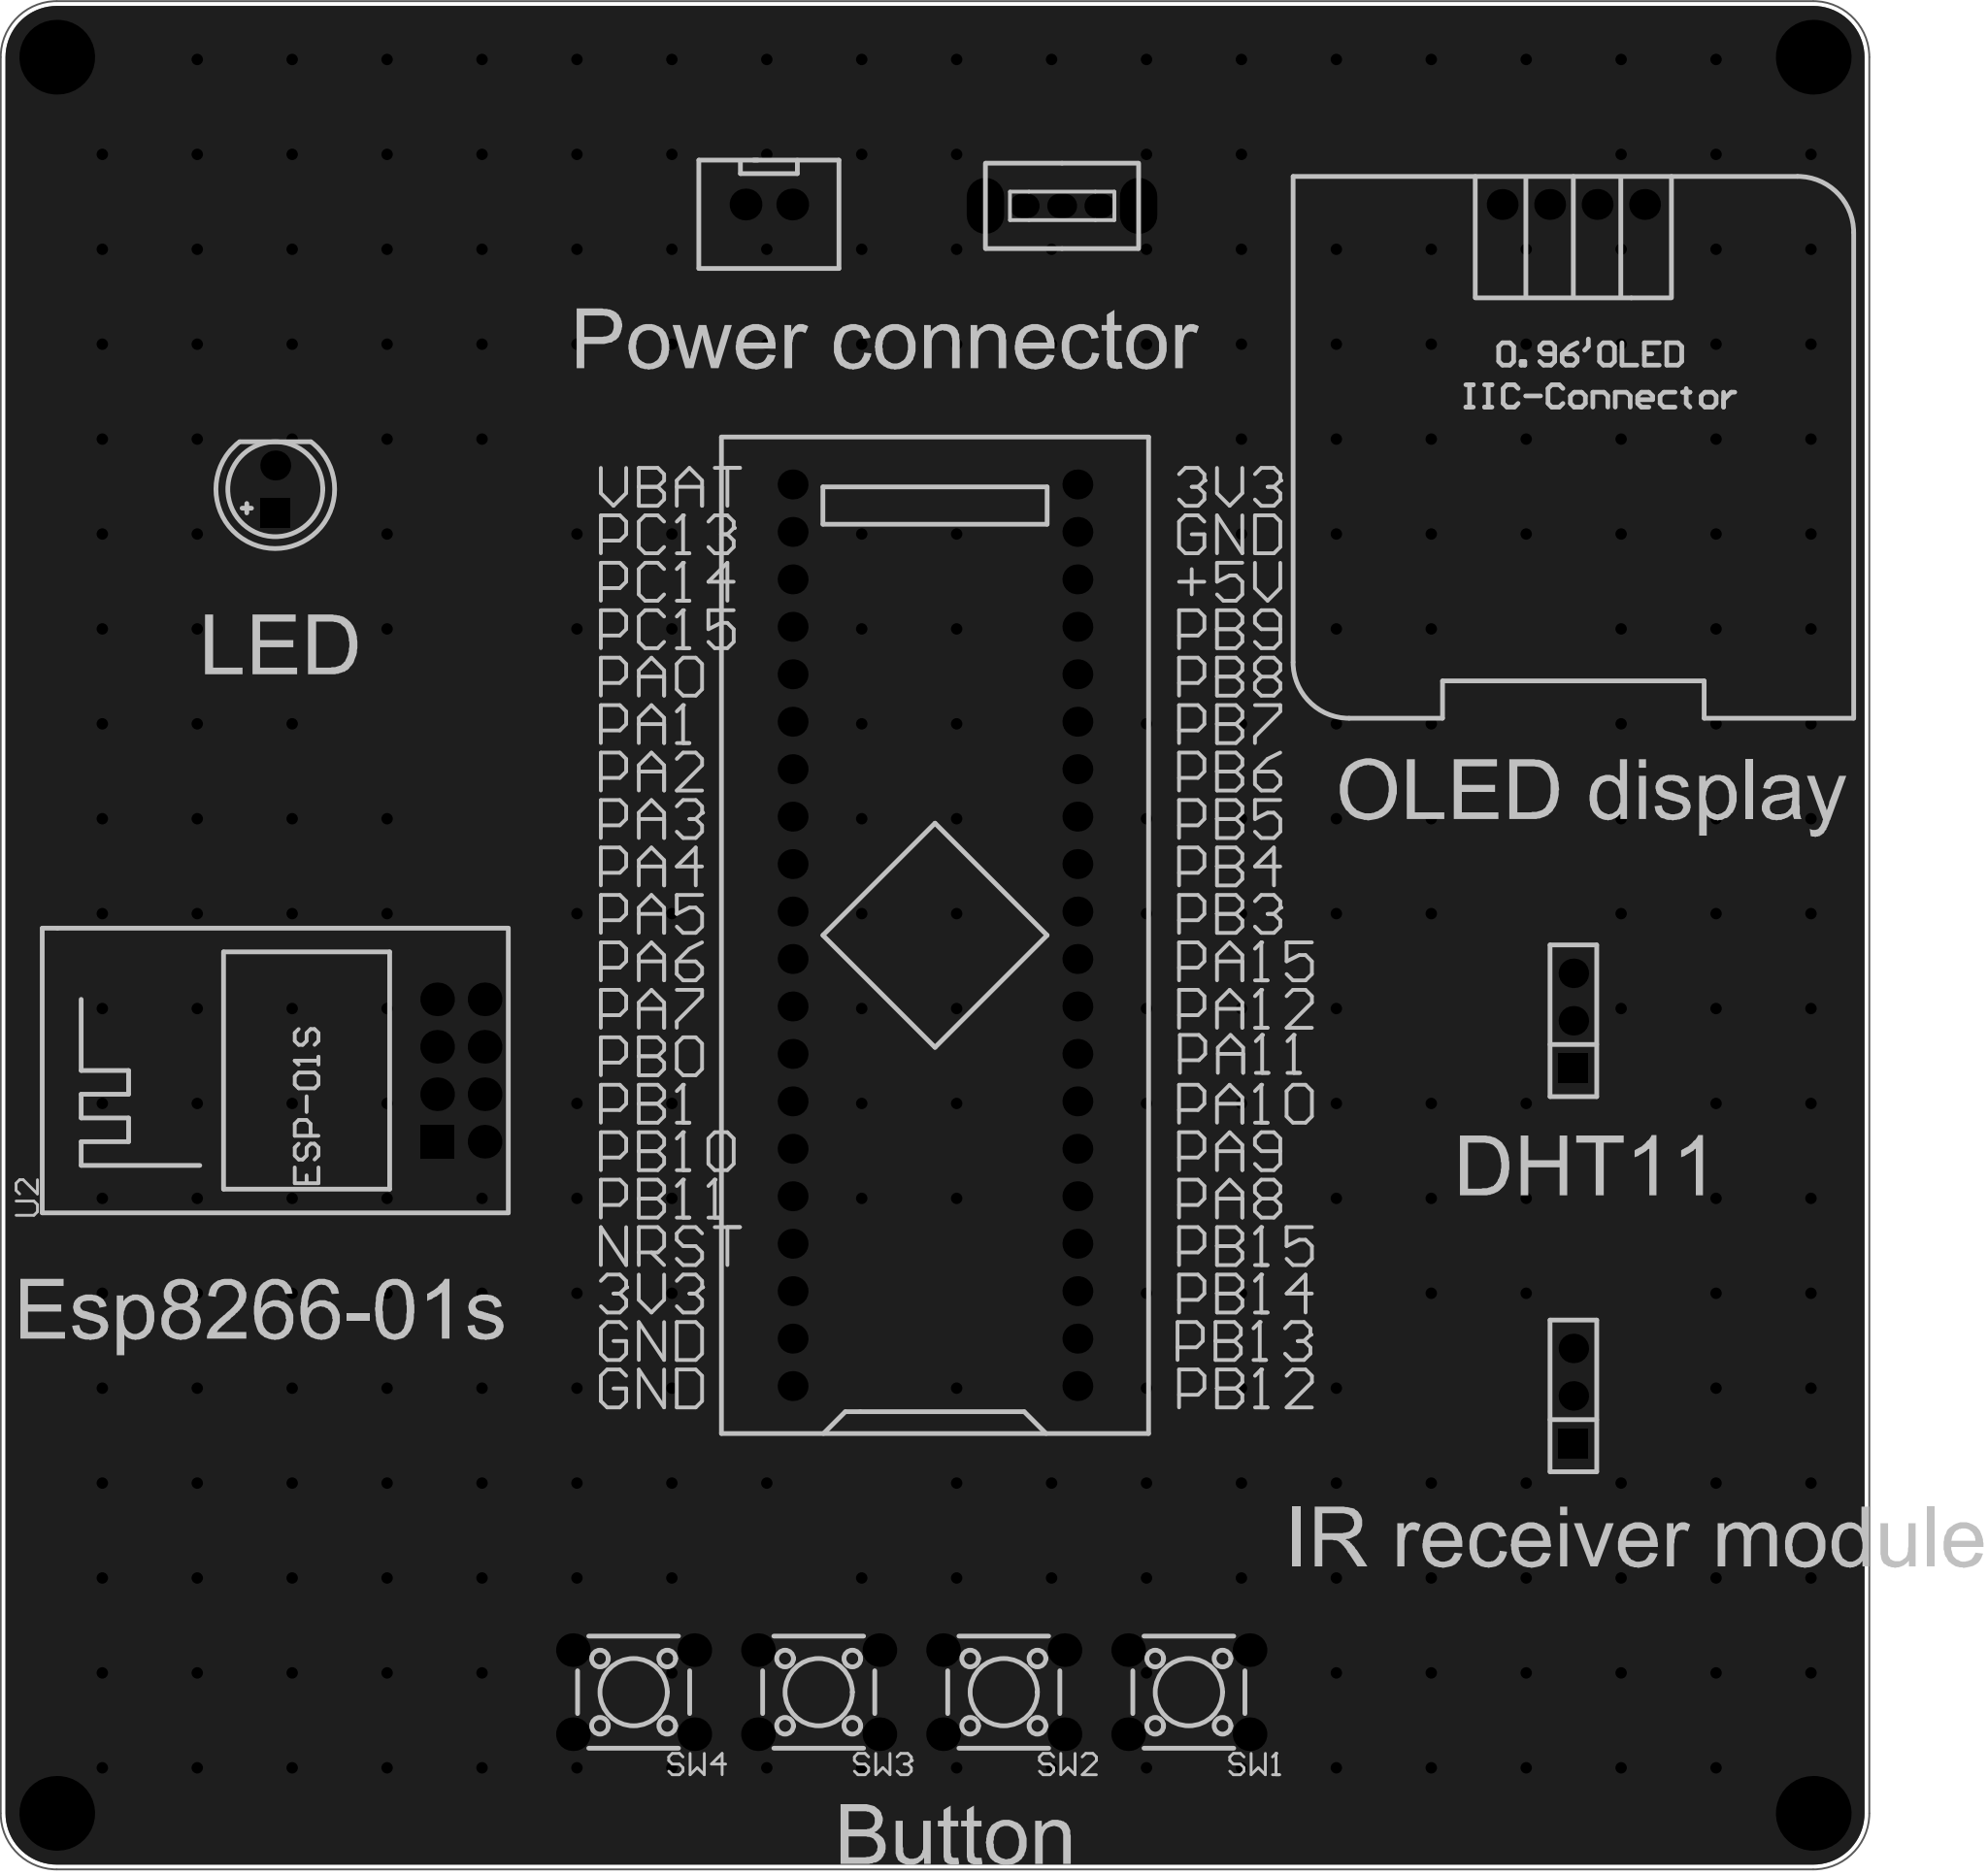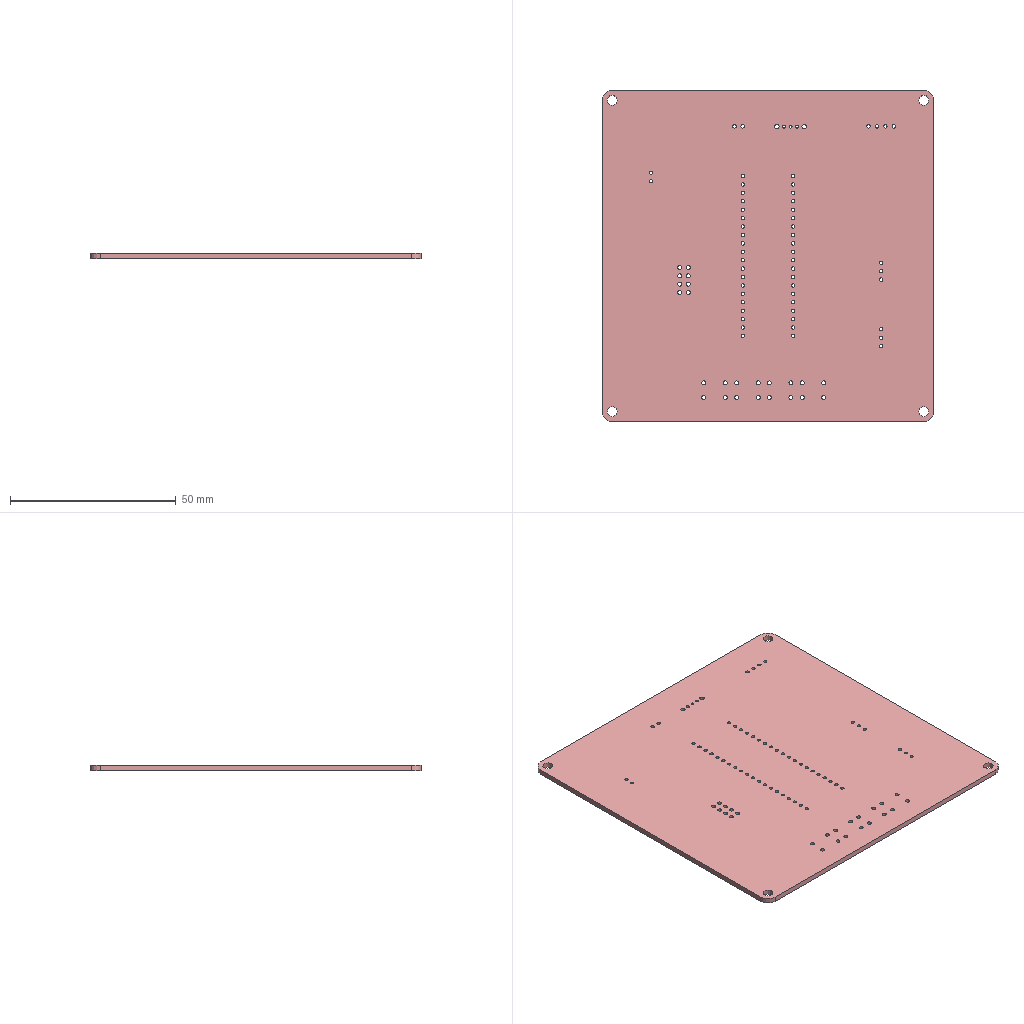Circuit board layout | Altium Designer | box 100 x 100 x 1.6 mm
Layer stack:
# Altium Designer layer stack of  (unit mm; dielectric type: 0 none, 1 core, 2 prepreg, 3 surface material)
index,name,kind,layer,copper_thickness_mm,dielectric_type,dielectric_thickness_mm,dielectric_material,dielectric_constant
0,Top Paste Mask Layer,other,,,,,,
1,Top Silkscreen Layer,other,,,,,,
2,Top Solder Mask Layer,dielectric,,,3,0.01,,3.3
3,Top Layer,copper,Top Layer,0.035,,,,
4,Dielectric1,dielectric,,,3,1.51,FR4,4.5
5,Bottom Layer,copper,Bottom Layer,0.035,,,,
6,Bottom Solder Mask Layer,dielectric,,,3,0.01,,3.3
7,Bottom Silkscreen Layer,other,,,,,,
8,Bottom Paste Mask Layer,other,,,,,,
# drill layer pairs: low layer,high layer
drill_pair,Top Layer,Bottom Layer
Part placement:
Designator,Comment,Layer,Footprint,Center-X(mm),Center-Y(mm),Rotation
U1,STM32F103C8T6-Card,TopLayer,CONN-TH_L53.3-W22.9_STM32F103C8T6-CARD,141.351,130.937,90
SW1,,TopLayer,SW-TH_4P-L6.0-W6.0-P4.50-LS6.5,154.936,90.424,180
SW2,,TopLayer,SW-TH_4P-L6.0-W6.0-P4.50-LS6.5,145.031,90.424,180
SW3,,TopLayer,SW-TH_4P-L6.0-W6.0-P4.50-LS6.5,135.127,90.424,180
SW4,,TopLayer,SW-TH_4P-L6.0-W6.0-P4.50-LS6.5,125.222,90.424,180
CN4,XH2.54*2P_THT,TopLayer,CONN-TH_2P-P2.50-XH2.54-2P,132.461,170.053,0
SW5,,TopLayer,拨动开关,148.148,169.978,180
H1,,TopLayer,HDR-TH_3P-P2.54-V-F,175.514,106.281,90
H3,,TopLayer,HDR-TH_3P-P2.54-V-F,175.514,126.36,90
LED1,,TopLayer,LED-TH_5mm,106.045,154.813,90
OLED1,,TopLayer,0.96OLED_4P,175.514,170.053,0
U2,ESP-01S,TopLayer,WIFIM-TH_ESP-01S,115.976,123.698,90
Pad and via stacks:
# Altium Designer via and pad stacks of  (unit mm). Each distinct definition once, with the count of objects using it.
# via: kind,start_layer,end_layer,hole_mm,diameter_mm,mode(0 simple;1 top-mid-bottom;2 full stack),diameter_per_layer,count,example_net
# pad: kind,layer,hole_mm,hole_type(0 round;1 square;2 slot),plating,top_size,top_shape(1 round;2 rect;3 octagon;9 rounded rect),mid_size,bottom_size,mode,footprint,size_per_layer,count,example
pad,Multi-Layer,3,0,plated,4x4,1,4x4,4x4,0,,,4,1
pad,Multi-Layer,1,0,plated,1.6x1.6,1,1.6x1.6,1.6x1.6,0,CONN-TH_L53.3-W22.9_STM32F103C8T6-CARD,,40,U1.1
pad,Multi-Layer,1.2,0,plated,1.8x1.8,1,1.8x1.8,1.8x1.8,0,SW-TH_4P-L6.0-W6.0-P4.50-LS6.5,,16,SW1.1
pad,Multi-Layer,1.05,0,plated,1.7x1.7,1,1.7x1.7,1.7x1.7,0,CONN-TH_2P-P2.50-XH2.54-2P,,2,CN4.2
pad,Multi-Layer,0.8992,0,plated,1.6x1.3,1,1.6x1.3,1.6x1.3,0,\u00B2\u00A6\u00B6\u00AF\u00BF\u00AA\u00B9\u00D8,,3,SW5.1
pad,Multi-Layer,1.3,0,plated,3x1.999,1,3x1.999,3x1.999,0,\u00B2\u00A6\u00B6\u00AF\u00BF\u00AA\u00B9\u00D8,,2,SW5.4
pad,Multi-Layer,1.02,0,plated,1.575x1.575,1,1.575x1.575,1.575x1.575,0,HDR-TH_3P-P2.54-V-F,,4,H1.3
pad,Multi-Layer,1.02,0,plated,1.575x1.575,2,1.575x1.575,1.575x1.575,0,HDR-TH_3P-P2.54-V-F,,2,H1.1
pad,Multi-Layer,1,0,plated,1.6x1.6,2,1.6x1.6,1.6x1.6,0,LED-TH_5mm,,1,LED1.1
pad,Multi-Layer,1,0,plated,1.6x1.6,1,1.6x1.6,1.6x1.6,0,LED-TH_5mm,,1,LED1.2
pad,Multi-Layer,1,0,plated,1.65x1.65,1,1.65x1.65,1.65x1.65,0,0.96OLED_4P,,4,OLED1.4
pad,Multi-Layer,1.2,0,plated,1.8x1.8,2,1.8x1.8,1.8x1.8,0,WIFIM-TH_ESP-01S,,1,U2.1
pad,Multi-Layer,1.2,0,plated,1.8x1.8,1,1.8x1.8,1.8x1.8,0,WIFIM-TH_ESP-01S,,7,U2.2
via,Top Layer,Bottom Layer,0.3048,0.61,0,,282,GND
Copper pours:
name,layer,net,type(0 solid;1 hatched;2 none)
Bottom Layer-GND,Bottom Layer,GND,0
Top Layer-GND,Top Layer,GND,0
Design rules, without the lines most boards share:
# Altium Designer design rules of  (exported by Altium Designer, unit mm)
# columns: name | kind | enabled | priority | scope1 | scope2 | descriptor | typed fields (field=value)
Copper_copperRegion_copperThickness1oz | 0 | disabled | 4 | All | All | Clearance Constraint (Gap=5.984mil) (Disabled)(All),(All) | gap=0.152
Copper_copperRegion_copperThickness1oz_1 | 63 | disabled | 4 | All | All | Board Clearance Constraint (Gap=0mil) (Disabled)(All) |
Copper_copperRegion_Copper_copperRegion | 0 | disabled | 5 | All | All | Clearance Constraint (Gap=5.984mil) (Disabled)(All),(All) | gap=0.152
Copper_copperRegion_Copper_copperRegion_1 | 63 | disabled | 5 | All | All | Board Clearance Constraint (Gap=0mil) (Disabled)(All) |
copperThickness1oz | 0 | enabled | 6 | All | All | Clearance Constraint (Gap=5.984mil) (All),(All) | gap=0.152
copperThickness1oz_1 | 63 | enabled | 6 | All | All | Board Clearance Constraint (Gap=0mil) (All) |
copperRegion_copperThickness1oz | 20 | disabled | 1 | All | All | Polygon Connect Rule(Relief Connect )(Conductor Width=10mil) (Relief Angle=90 Angle) (Entries=4) (Air Gap Width=10mil) (Disabled)(All),(All) | connect_style(0=relief,1=direct,2=none)=0 relief_conductor_width=0.254 relief_entries=4
copperRegion_Copper_copperRegion | 20 | disabled | 2 | All | All | Polygon Connect Rule(Relief Connect )(Conductor Width=10mil) (Relief Angle=90 Angle) (Entries=4) (Air Gap Width=10mil) (Disabled)(All),(All) | connect_style(0=relief,1=direct,2=none)=0 relief_conductor_width=0.254 relief_entries=4
copperRegion | 20 | enabled | 3 | All | All | Polygon Connect Rule(Relief Connect )(Conductor Width=10mil) (Relief Angle=90 Angle) (Entries=4) (Air Gap Width=10mil) (All),(All) | connect_style(0=relief,1=direct,2=none)=0 relief_conductor_width=0.254 relief_entries=4